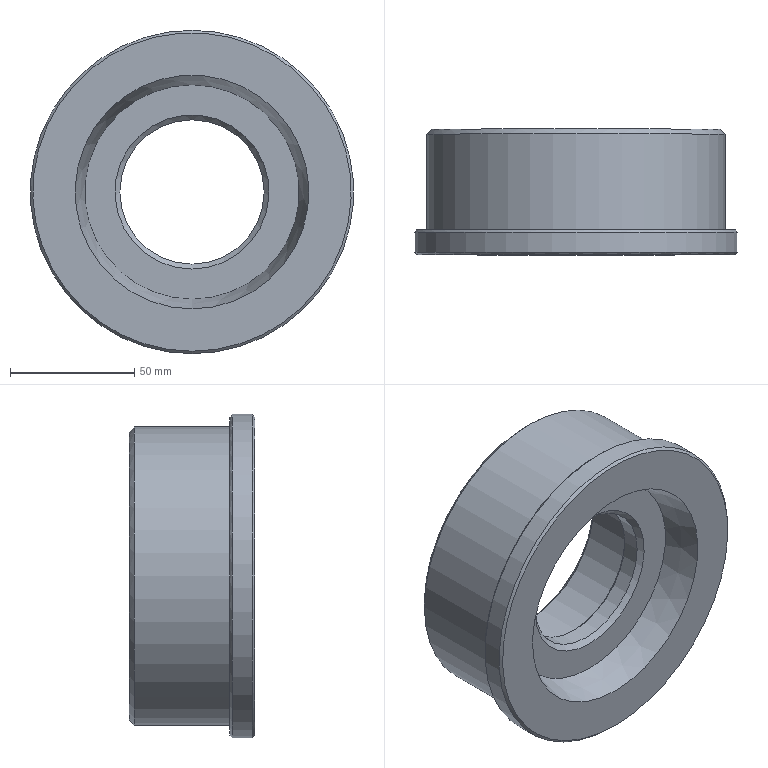Part | NX | features BREP 1, DATUM_CSYS 1 | 1 solid | 16 faces | box 130 x 50.5 x 130 mm | volume 363881 mm3 | cone 7 | plane 5 | cylinder 4 | commonest cylinder face diameters 58 x1 72 x1 120 x1 130 x1
STEP:
#1=CARTESIAN_POINT('',(160.,-671.5,143.));
#2=VERTEX_POINT('',#1);
#3=CARTESIAN_POINT('',(160.,-671.5,179.));
#4=DIRECTION('',(0.,-1.,0.));
#5=DIRECTION('',(0.,0.,-1.));
#6=AXIS2_PLACEMENT_3D('',#3,#4,#5);
#7=CIRCLE('',#6,36.);
#8=EDGE_CURVE('',#2,#2,#7,.T.);
#9=ORIENTED_EDGE('',*,*,#8,.T.);
#10=EDGE_LOOP('',(#9));
#11=FACE_BOUND('',#10,.T.);
#12=CARTESIAN_POINT('',(160.,-647.5,143.));
#13=VERTEX_POINT('',#12);
#14=CARTESIAN_POINT('',(160.,-647.5,179.));
#15=DIRECTION('',(0.,-1.,0.));
#16=DIRECTION('',(0.,0.,-1.));
#17=AXIS2_PLACEMENT_3D('',#14,#15,#16);
#18=CIRCLE('',#17,36.);
#19=EDGE_CURVE('',#13,#13,#18,.T.);
#20=ORIENTED_EDGE('',*,*,#19,.F.);
#21=EDGE_LOOP('',(#20));
#22=FACE_BOUND('',#21,.T.);
#23=CARTESIAN_POINT('',(160.,-685.,179.));
#24=DIRECTION('',(0.,-1.,0.));
#25=DIRECTION('',(0.,0.,-1.));
#26=AXIS2_PLACEMENT_3D('',#23,#24,#25);
#27=CYLINDRICAL_SURFACE('',#26,36.);
#28=ADVANCED_FACE('',(#11,#22),#27,.F.);
#29=CARTESIAN_POINT('',(160.,-671.5,149.));
#30=VERTEX_POINT('',#29);
#31=CARTESIAN_POINT('',(160.,-671.5,179.));
#32=DIRECTION('',(0.,-1.,0.));
#33=DIRECTION('',(0.,0.,-1.));
#34=AXIS2_PLACEMENT_3D('',#31,#32,#33);
#35=CIRCLE('',#34,30.);
#36=EDGE_CURVE('',#30,#30,#35,.T.);
#37=ORIENTED_EDGE('',*,*,#36,.T.);
#38=EDGE_LOOP('',(#37));
#39=FACE_BOUND('',#38,.T.);
#40=ORIENTED_EDGE('',*,*,#8,.F.);
#41=EDGE_LOOP('',(#40));
#42=FACE_BOUND('',#41,.T.);
#43=CARTESIAN_POINT('',(124.,-671.5,179.));
#44=DIRECTION('',(0.,1.,0.));
#45=DIRECTION('',(0.,0.,1.));
#46=AXIS2_PLACEMENT_3D('',#43,#44,#45);
#47=PLANE('',#46);
#48=ADVANCED_FACE('',(#39,#42),#47,.T.);
#49=CARTESIAN_POINT('',(160.,-672.5,150.));
#50=VERTEX_POINT('',#49);
#51=CARTESIAN_POINT('',(160.,-672.5,179.));
#52=DIRECTION('',(0.,-1.,0.));
#53=DIRECTION('',(0.,0.,-1.));
#54=AXIS2_PLACEMENT_3D('',#51,#52,#53);
#55=CIRCLE('',#54,29.);
#56=EDGE_CURVE('',#50,#50,#55,.T.);
#57=ORIENTED_EDGE('',*,*,#56,.T.);
#58=EDGE_LOOP('',(#57));
#59=FACE_BOUND('',#58,.T.);
#60=ORIENTED_EDGE('',*,*,#36,.F.);
#61=EDGE_LOOP('',(#60));
#62=FACE_BOUND('',#61,.T.);
#63=CARTESIAN_POINT('',(160.,-671.5,179.));
#64=DIRECTION('',(0.,1.,0.));
#65=DIRECTION('',(0.,0.,1.));
#66=AXIS2_PLACEMENT_3D('',#63,#64,#65);
#67=CONICAL_SURFACE('',#66,30.,0.7854);
#68=ADVANCED_FACE('',(#59,#62),#67,.F.);
#69=CARTESIAN_POINT('',(160.,-679.5,150.));
#70=VERTEX_POINT('',#69);
#71=CARTESIAN_POINT('',(160.,-679.5,179.));
#72=DIRECTION('',(0.,-1.,0.));
#73=DIRECTION('',(0.,0.,-1.));
#74=AXIS2_PLACEMENT_3D('',#71,#72,#73);
#75=CIRCLE('',#74,29.);
#76=EDGE_CURVE('',#70,#70,#75,.T.);
#77=ORIENTED_EDGE('',*,*,#76,.T.);
#78=EDGE_LOOP('',(#77));
#79=FACE_BOUND('',#78,.T.);
#80=ORIENTED_EDGE('',*,*,#56,.F.);
#81=EDGE_LOOP('',(#80));
#82=FACE_BOUND('',#81,.T.);
#83=CARTESIAN_POINT('',(160.,-685.,179.));
#84=DIRECTION('',(0.,-1.,0.));
#85=DIRECTION('',(0.,0.,-1.));
#86=AXIS2_PLACEMENT_3D('',#83,#84,#85);
#87=CYLINDRICAL_SURFACE('',#86,29.);
#88=ADVANCED_FACE('',(#79,#82),#87,.F.);
#89=CARTESIAN_POINT('',(160.,-681.5,148.));
#90=VERTEX_POINT('',#89);
#91=CARTESIAN_POINT('',(160.,-681.5,179.));
#92=DIRECTION('',(0.,-1.,0.));
#93=DIRECTION('',(0.,0.,-1.));
#94=AXIS2_PLACEMENT_3D('',#91,#92,#93);
#95=CIRCLE('',#94,31.);
#96=EDGE_CURVE('',#90,#90,#95,.T.);
#97=ORIENTED_EDGE('',*,*,#96,.T.);
#98=EDGE_LOOP('',(#97));
#99=FACE_BOUND('',#98,.T.);
#100=ORIENTED_EDGE('',*,*,#76,.F.);
#101=EDGE_LOOP('',(#100));
#102=FACE_BOUND('',#101,.T.);
#103=CARTESIAN_POINT('',(160.,-679.5,179.));
#104=DIRECTION('',(0.,-1.,0.));
#105=DIRECTION('',(0.,0.,-1.));
#106=AXIS2_PLACEMENT_3D('',#103,#104,#105);
#107=CONICAL_SURFACE('',#106,29.,0.7854);
#108=ADVANCED_FACE('',(#99,#102),#107,.F.);
#109=CARTESIAN_POINT('',(160.,-681.5,135.885));
#110=VERTEX_POINT('',#109);
#111=CARTESIAN_POINT('',(160.,-681.5,179.));
#112=DIRECTION('',(0.,-1.,0.));
#113=DIRECTION('',(0.,0.,-1.));
#114=AXIS2_PLACEMENT_3D('',#111,#112,#113);
#115=CIRCLE('',#114,43.115);
#116=EDGE_CURVE('',#110,#110,#115,.T.);
#117=ORIENTED_EDGE('',*,*,#116,.T.);
#118=EDGE_LOOP('',(#117));
#119=FACE_BOUND('',#118,.T.);
#120=ORIENTED_EDGE('',*,*,#96,.F.);
#121=EDGE_LOOP('',(#120));
#122=FACE_BOUND('',#121,.T.);
#123=CARTESIAN_POINT('',(129.,-681.5,179.));
#124=DIRECTION('',(0.,-1.,0.));
#125=DIRECTION('',(0.,0.,-1.));
#126=AXIS2_PLACEMENT_3D('',#123,#124,#125);
#127=PLANE('',#126);
#128=ADVANCED_FACE('',(#119,#122),#127,.T.);
#129=CARTESIAN_POINT('',(160.,-696.,132.));
#130=VERTEX_POINT('',#129);
#131=CARTESIAN_POINT('',(160.,-696.,179.));
#132=DIRECTION('',(0.,-1.,0.));
#133=DIRECTION('',(0.,0.,-1.));
#134=AXIS2_PLACEMENT_3D('',#131,#132,#133);
#135=CIRCLE('',#134,47.);
#136=EDGE_CURVE('',#130,#130,#135,.T.);
#137=ORIENTED_EDGE('',*,*,#136,.T.);
#138=EDGE_LOOP('',(#137));
#139=FACE_BOUND('',#138,.T.);
#140=ORIENTED_EDGE('',*,*,#116,.F.);
#141=EDGE_LOOP('',(#140));
#142=FACE_BOUND('',#141,.T.);
#143=CARTESIAN_POINT('',(160.,-681.5,179.));
#144=DIRECTION('',(0.,-1.,0.));
#145=DIRECTION('',(0.,0.,-1.));
#146=AXIS2_PLACEMENT_3D('',#143,#144,#145);
#147=CONICAL_SURFACE('',#146,43.115,0.2618);
#148=ADVANCED_FACE('',(#139,#142),#147,.F.);
#149=CARTESIAN_POINT('',(160.,-696.,115.));
#150=VERTEX_POINT('',#149);
#151=CARTESIAN_POINT('',(160.,-696.,179.));
#152=DIRECTION('',(0.,-1.,0.));
#153=DIRECTION('',(0.,0.,-1.));
#154=AXIS2_PLACEMENT_3D('',#151,#152,#153);
#155=CIRCLE('',#154,64.);
#156=EDGE_CURVE('',#150,#150,#155,.T.);
#157=ORIENTED_EDGE('',*,*,#156,.T.);
#158=EDGE_LOOP('',(#157));
#159=FACE_BOUND('',#158,.T.);
#160=ORIENTED_EDGE('',*,*,#136,.F.);
#161=EDGE_LOOP('',(#160));
#162=FACE_BOUND('',#161,.T.);
#163=CARTESIAN_POINT('',(113.,-696.,179.));
#164=DIRECTION('',(0.,-1.,0.));
#165=DIRECTION('',(0.,0.,-1.));
#166=AXIS2_PLACEMENT_3D('',#163,#164,#165);
#167=PLANE('',#166);
#168=ADVANCED_FACE('',(#159,#162),#167,.T.);
#169=CARTESIAN_POINT('',(160.,-695.,114.));
#170=VERTEX_POINT('',#169);
#171=CARTESIAN_POINT('',(160.,-695.,179.));
#172=DIRECTION('',(0.,-1.,0.));
#173=DIRECTION('',(0.,0.,-1.));
#174=AXIS2_PLACEMENT_3D('',#171,#172,#173);
#175=CIRCLE('',#174,65.);
#176=EDGE_CURVE('',#170,#170,#175,.T.);
#177=ORIENTED_EDGE('',*,*,#176,.T.);
#178=EDGE_LOOP('',(#177));
#179=FACE_BOUND('',#178,.T.);
#180=ORIENTED_EDGE('',*,*,#156,.F.);
#181=EDGE_LOOP('',(#180));
#182=FACE_BOUND('',#181,.T.);
#183=CARTESIAN_POINT('',(160.,-696.,179.));
#184=DIRECTION('',(0.,1.,0.));
#185=DIRECTION('',(0.,0.,1.));
#186=AXIS2_PLACEMENT_3D('',#183,#184,#185);
#187=CONICAL_SURFACE('',#186,64.,0.7854);
#188=ADVANCED_FACE('',(#179,#182),#187,.T.);
#189=CARTESIAN_POINT('',(160.,-687.,114.));
#190=VERTEX_POINT('',#189);
#191=CARTESIAN_POINT('',(160.,-687.,179.));
#192=DIRECTION('',(0.,-1.,0.));
#193=DIRECTION('',(0.,0.,-1.));
#194=AXIS2_PLACEMENT_3D('',#191,#192,#193);
#195=CIRCLE('',#194,65.);
#196=EDGE_CURVE('',#190,#190,#195,.T.);
#197=ORIENTED_EDGE('',*,*,#196,.T.);
#198=EDGE_LOOP('',(#197));
#199=FACE_BOUND('',#198,.T.);
#200=ORIENTED_EDGE('',*,*,#176,.F.);
#201=EDGE_LOOP('',(#200));
#202=FACE_BOUND('',#201,.T.);
#203=CARTESIAN_POINT('',(160.,-685.,179.));
#204=DIRECTION('',(0.,-1.,0.));
#205=DIRECTION('',(0.,0.,-1.));
#206=AXIS2_PLACEMENT_3D('',#203,#204,#205);
#207=CYLINDRICAL_SURFACE('',#206,65.);
#208=ADVANCED_FACE('',(#199,#202),#207,.T.);
#209=CARTESIAN_POINT('',(160.,-686.,115.));
#210=VERTEX_POINT('',#209);
#211=CARTESIAN_POINT('',(160.,-686.,179.));
#212=DIRECTION('',(0.,-1.,0.));
#213=DIRECTION('',(0.,0.,-1.));
#214=AXIS2_PLACEMENT_3D('',#211,#212,#213);
#215=CIRCLE('',#214,64.);
#216=EDGE_CURVE('',#210,#210,#215,.T.);
#217=ORIENTED_EDGE('',*,*,#216,.T.);
#218=EDGE_LOOP('',(#217));
#219=FACE_BOUND('',#218,.T.);
#220=ORIENTED_EDGE('',*,*,#196,.F.);
#221=EDGE_LOOP('',(#220));
#222=FACE_BOUND('',#221,.T.);
#223=CARTESIAN_POINT('',(160.,-687.,179.));
#224=DIRECTION('',(0.,-1.,0.));
#225=DIRECTION('',(0.,0.,-1.));
#226=AXIS2_PLACEMENT_3D('',#223,#224,#225);
#227=CONICAL_SURFACE('',#226,65.,0.7854);
#228=ADVANCED_FACE('',(#219,#222),#227,.T.);
#229=CARTESIAN_POINT('',(160.,-686.,119.));
#230=VERTEX_POINT('',#229);
#231=CARTESIAN_POINT('',(160.,-686.,179.));
#232=DIRECTION('',(0.,-1.,0.));
#233=DIRECTION('',(0.,0.,-1.));
#234=AXIS2_PLACEMENT_3D('',#231,#232,#233);
#235=CIRCLE('',#234,60.);
#236=EDGE_CURVE('',#230,#230,#235,.T.);
#237=ORIENTED_EDGE('',*,*,#236,.T.);
#238=EDGE_LOOP('',(#237));
#239=FACE_BOUND('',#238,.T.);
#240=ORIENTED_EDGE('',*,*,#216,.F.);
#241=EDGE_LOOP('',(#240));
#242=FACE_BOUND('',#241,.T.);
#243=CARTESIAN_POINT('',(96.,-686.,179.));
#244=DIRECTION('',(0.,1.,0.));
#245=DIRECTION('',(0.,0.,1.));
#246=AXIS2_PLACEMENT_3D('',#243,#244,#245);
#247=PLANE('',#246);
#248=ADVANCED_FACE('',(#239,#242),#247,.T.);
#249=CARTESIAN_POINT('',(160.,-647.5,119.));
#250=VERTEX_POINT('',#249);
#251=CARTESIAN_POINT('',(160.,-647.5,179.));
#252=DIRECTION('',(0.,-1.,0.));
#253=DIRECTION('',(0.,0.,-1.));
#254=AXIS2_PLACEMENT_3D('',#251,#252,#253);
#255=CIRCLE('',#254,60.);
#256=EDGE_CURVE('',#250,#250,#255,.T.);
#257=ORIENTED_EDGE('',*,*,#256,.T.);
#258=EDGE_LOOP('',(#257));
#259=FACE_BOUND('',#258,.T.);
#260=ORIENTED_EDGE('',*,*,#236,.F.);
#261=EDGE_LOOP('',(#260));
#262=FACE_BOUND('',#261,.T.);
#263=CARTESIAN_POINT('',(160.,-685.,179.));
#264=DIRECTION('',(0.,-1.,0.));
#265=DIRECTION('',(0.,0.,-1.));
#266=AXIS2_PLACEMENT_3D('',#263,#264,#265);
#267=CYLINDRICAL_SURFACE('',#266,60.);
#268=ADVANCED_FACE('',(#259,#262),#267,.T.);
#269=CARTESIAN_POINT('',(160.,-645.5,121.));
#270=VERTEX_POINT('',#269);
#271=CARTESIAN_POINT('',(160.,-645.5,179.));
#272=DIRECTION('',(0.,-1.,0.));
#273=DIRECTION('',(0.,0.,-1.));
#274=AXIS2_PLACEMENT_3D('',#271,#272,#273);
#275=CIRCLE('',#274,58.);
#276=EDGE_CURVE('',#270,#270,#275,.T.);
#277=ORIENTED_EDGE('',*,*,#276,.T.);
#278=EDGE_LOOP('',(#277));
#279=FACE_BOUND('',#278,.T.);
#280=ORIENTED_EDGE('',*,*,#256,.F.);
#281=EDGE_LOOP('',(#280));
#282=FACE_BOUND('',#281,.T.);
#283=CARTESIAN_POINT('',(160.,-647.5,179.));
#284=DIRECTION('',(0.,-1.,0.));
#285=DIRECTION('',(0.,0.,-1.));
#286=AXIS2_PLACEMENT_3D('',#283,#284,#285);
#287=CONICAL_SURFACE('',#286,60.,0.7854);
#288=ADVANCED_FACE('',(#279,#282),#287,.T.);
#289=CARTESIAN_POINT('',(160.,-645.5,141.));
#290=VERTEX_POINT('',#289);
#291=CARTESIAN_POINT('',(160.,-645.5,179.));
#292=DIRECTION('',(0.,-1.,0.));
#293=DIRECTION('',(0.,0.,-1.));
#294=AXIS2_PLACEMENT_3D('',#291,#292,#293);
#295=CIRCLE('',#294,38.);
#296=EDGE_CURVE('',#290,#290,#295,.T.);
#297=ORIENTED_EDGE('',*,*,#296,.T.);
#298=EDGE_LOOP('',(#297));
#299=FACE_BOUND('',#298,.T.);
#300=ORIENTED_EDGE('',*,*,#276,.F.);
#301=EDGE_LOOP('',(#300));
#302=FACE_BOUND('',#301,.T.);
#303=CARTESIAN_POINT('',(102.,-645.5,179.));
#304=DIRECTION('',(0.,1.,0.));
#305=DIRECTION('',(0.,0.,1.));
#306=AXIS2_PLACEMENT_3D('',#303,#304,#305);
#307=PLANE('',#306);
#308=ADVANCED_FACE('',(#299,#302),#307,.T.);
#309=ORIENTED_EDGE('',*,*,#19,.T.);
#310=EDGE_LOOP('',(#309));
#311=FACE_BOUND('',#310,.T.);
#312=ORIENTED_EDGE('',*,*,#296,.F.);
#313=EDGE_LOOP('',(#312));
#314=FACE_BOUND('',#313,.T.);
#315=CARTESIAN_POINT('',(160.,-645.5,179.));
#316=DIRECTION('',(0.,1.,0.));
#317=DIRECTION('',(0.,0.,1.));
#318=AXIS2_PLACEMENT_3D('',#315,#316,#317);
#319=CONICAL_SURFACE('',#318,38.,0.7854);
#320=ADVANCED_FACE('',(#311,#314),#319,.F.);
#321=CLOSED_SHELL('',(#28,#48,#68,#88,#108,#128,#148,#168,#188,#208,#228,#248,#268,#288,#308,#320));
#322=MANIFOLD_SOLID_BREP('',#321);
#323=(LENGTH_UNIT()NAMED_UNIT(*)SI_UNIT(.MILLI.,.METRE.));
#324=UNCERTAINTY_MEASURE_WITH_UNIT(LENGTH_MEASURE(0.00001),#323,'','');
#325=(NAMED_UNIT(*)PLANE_ANGLE_UNIT()SI_UNIT($,.RADIAN.));
#326=(NAMED_UNIT(*)SI_UNIT($,.STERADIAN.)SOLID_ANGLE_UNIT());
#327=(GEOMETRIC_REPRESENTATION_CONTEXT(3)GLOBAL_UNCERTAINTY_ASSIGNED_CONTEXT((#324))GLOBAL_UNIT_ASSIGNED_CONTEXT((#323,#325,#326))REPRESENTATION_CONTEXT('',''));
#328=ADVANCED_BREP_SHAPE_REPRESENTATION('',(#322),#327);